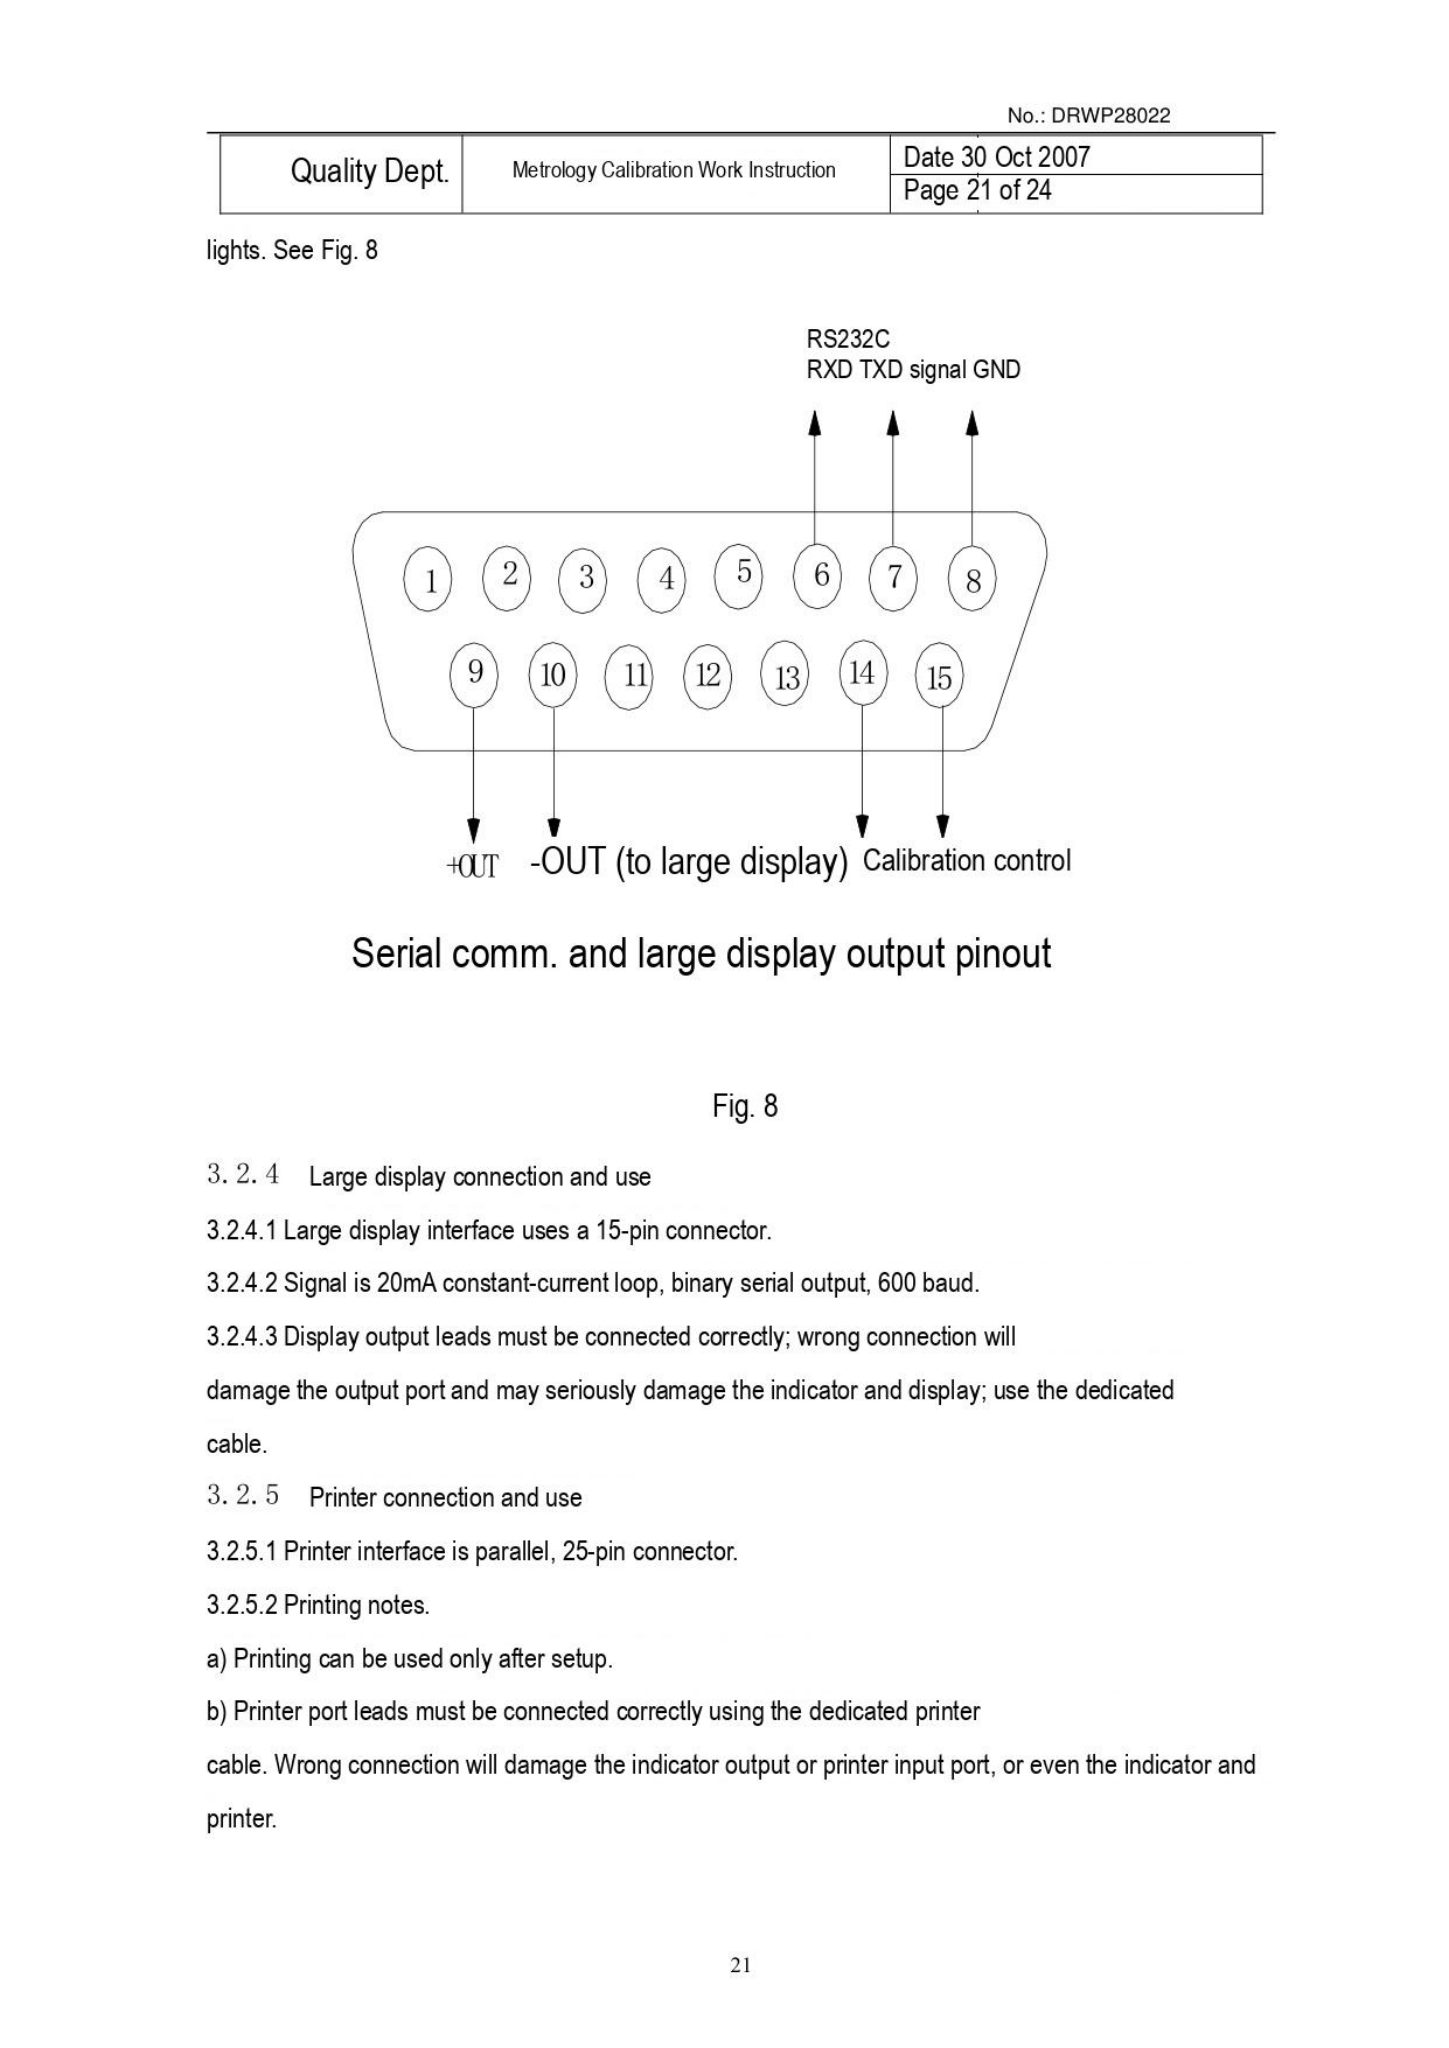No.: DRWP28022

| Quality Dept. | Metrology Calibration Work Instruction | Date 30 Oct 2007 |
|---|---|---|
| | | Page 21 of 24 |

lights. See Fig. 8

RS232C
RXD TXD signal GND

1 2 3 4 5 6 7 8
9 10 11 12 13 14 15

+OUT -OUT (to large display) Calibration control

Serial comm. and large display output pinout

Fig. 8

3. 2. 4 Large display connection and use

3.2.4.1 Large display interface uses a 15-pin connector.

3.2.4.2 Signal is 20mA constant-current loop, binary serial output, 600 baud.

3.2.4.3 Display output leads must be connected correctly; wrong connection will damage the output port and may seriously damage the indicator and display; use the dedicated cable.

3. 2. 5 Printer connection and use

3.2.5.1 Printer interface is parallel, 25-pin connector.

3.2.5.2 Printing notes.

a) Printing can be used only after setup.

b) Printer port leads must be connected correctly using the dedicated printer cable. Wrong connection will damage the indicator output or printer input port, or even the indicator and printer.

21
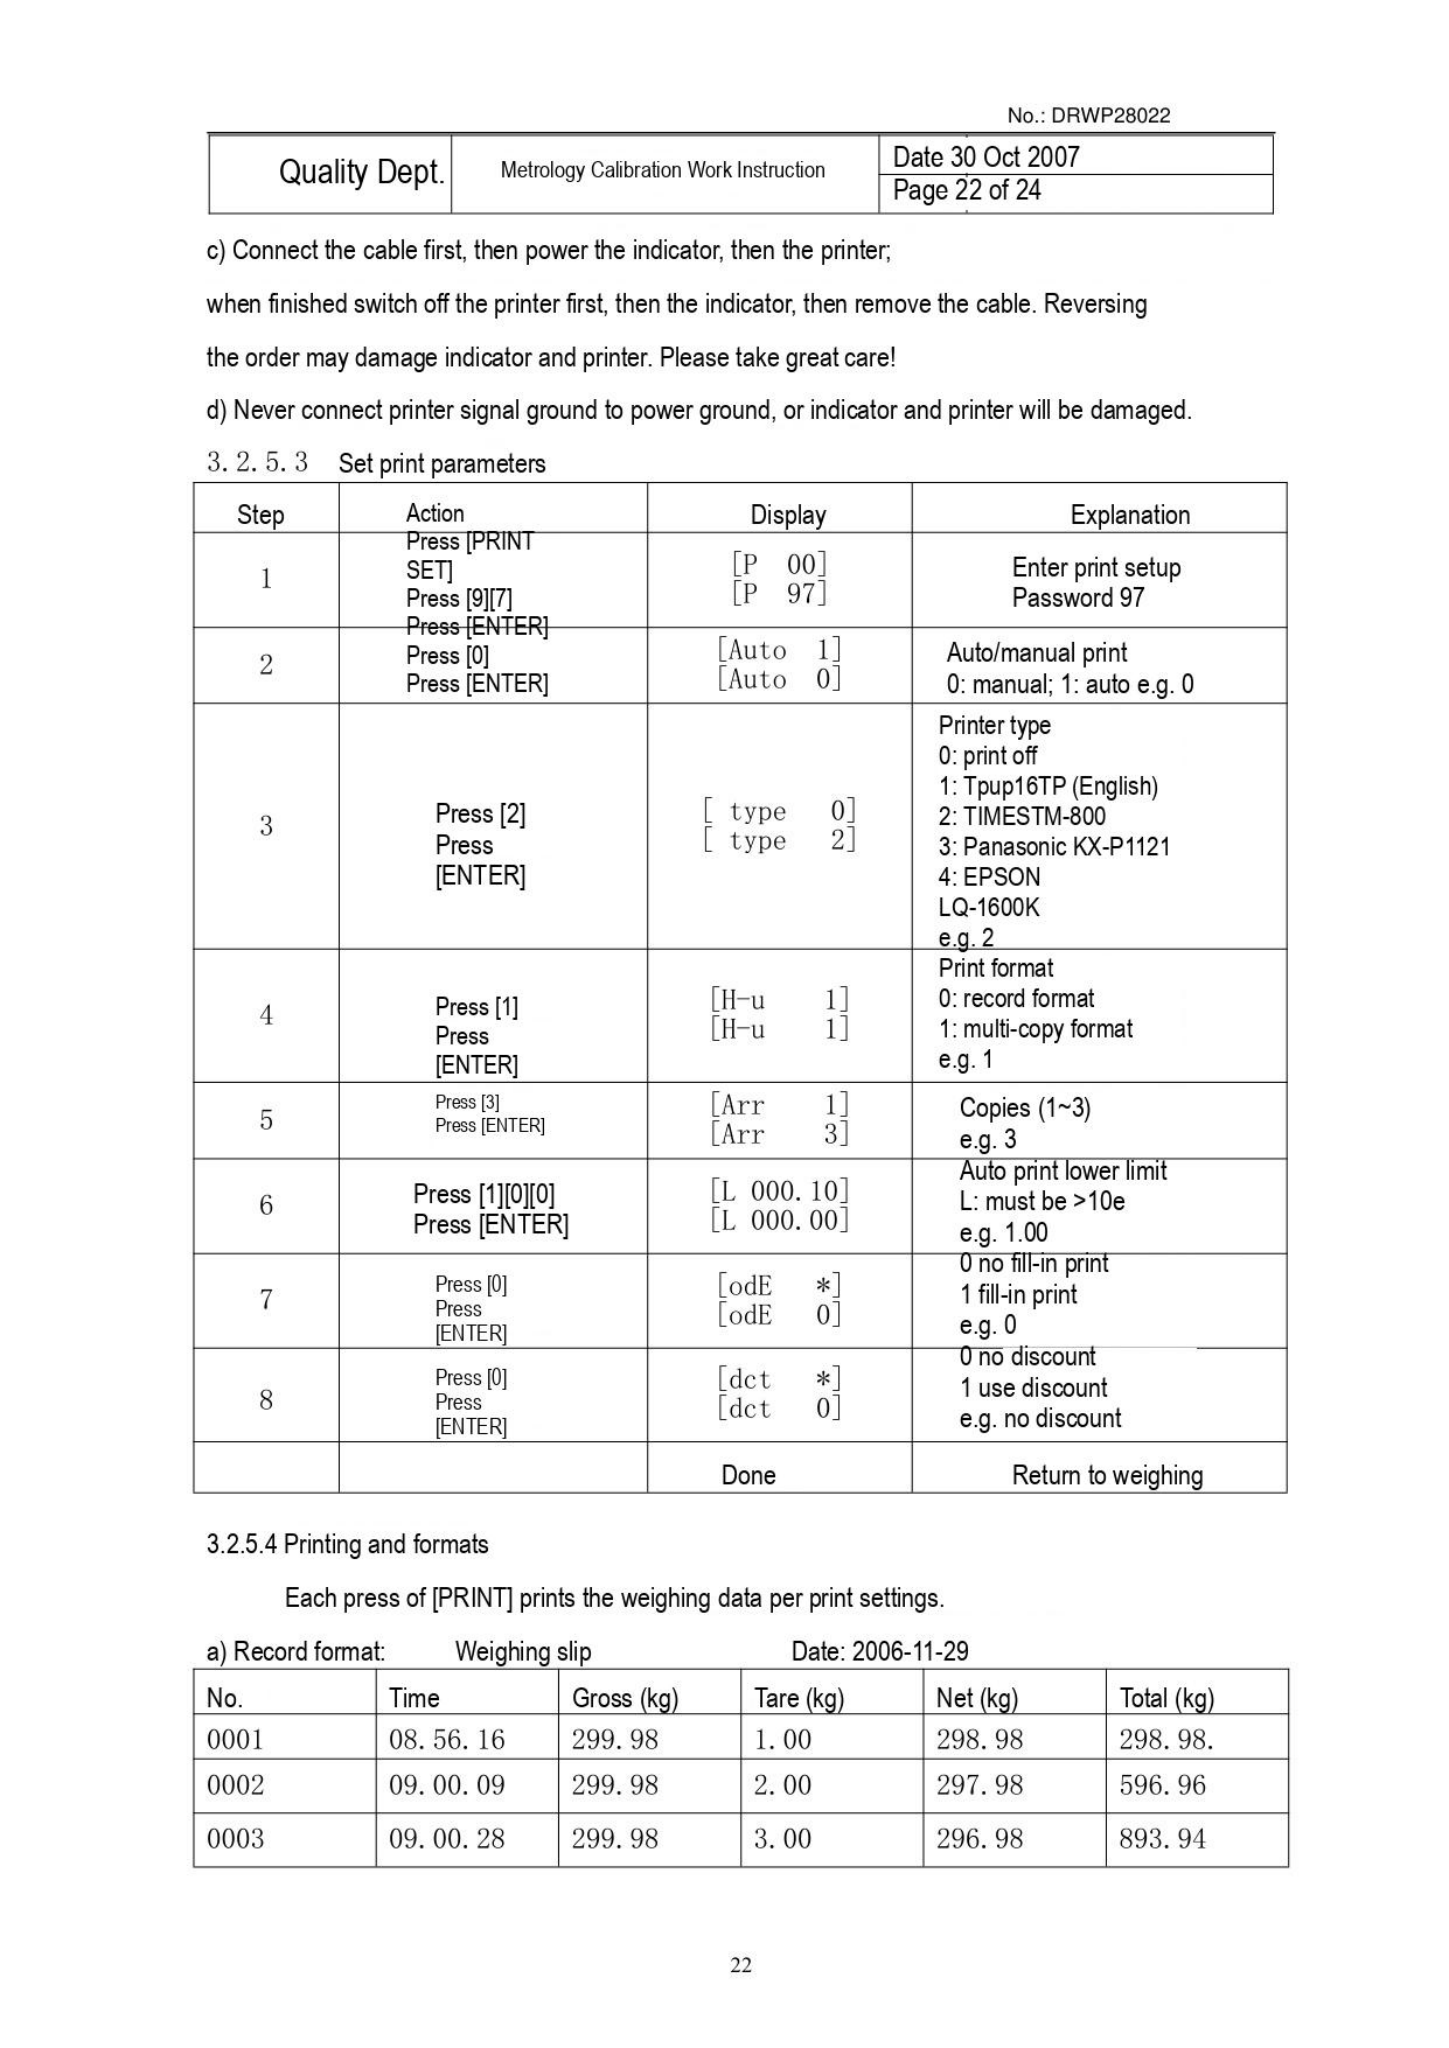No.: DRWP28022

| Quality Dept. | Metrology Calibration Work Instruction | Date 30 Oct 2007<br>Page 22 of 24 |
|---|---|---|

c) Connect the cable first, then power the indicator, then the printer;

when finished switch off the printer first, then the indicator, then remove the cable. Reversing

the order may damage indicator and printer. Please take great care!

d) Never connect printer signal ground to power ground, or indicator and printer will be damaged.

3. 2. 5. 3 Set print parameters

| Step | Action | Display | Explanation |
|---|---|---|---|
| 1 | Press [PRINT SET]<br>Press [9][7]<br>Press [ENTER] | [P 00]<br>[P 97] | Enter print setup<br>Password 97 |
| 2 | Press [0]<br>Press [ENTER] | [Auto 1]<br>[Auto 0] | Auto/manual print<br>0: manual; 1: auto e.g. 0 |
| 3 | Press [2]<br>Press [ENTER] | [ type 0]<br>[ type 2] | Printer type<br>0: print off<br>1: Tpup16TP (English)<br>2: TIMESTM-800<br>3: Panasonic KX-P1121<br>4: EPSON LQ-1600K<br>e.g. 2 |
| 4 | Press [1]<br>Press [ENTER] | [H-u 1]<br>[H-u 1] | Print format<br>0: record format<br>1: multi-copy format<br>e.g. 1 |
| 5 | Press [3]<br>Press [ENTER] | [Arr 1]<br>[Arr 3] | Copies (1~3)<br>e.g. 3 |
| 6 | Press [1][0][0]<br>Press [ENTER] | [L 000. 10]<br>[L 000. 00] | Auto print lower limit<br>L: must be >10e<br>e.g. 1.00 |
| 7 | Press [0]<br>Press [ENTER] | [odE *]<br>[odE 0] | 0 no fill-in print<br>1 fill-in print<br>e.g. 0 |
| 8 | Press [0]<br>Press [ENTER] | [dct *]<br>[dct 0] | 0 no discount<br>1 use discount<br>e.g. no discount |
| | | Done | Return to weighing |

3.2.5.4 Printing and formats

Each press of [PRINT] prints the weighing data per print settings.

a) Record format: Weighing slip Date: 2006-11-29

| No. | Time | Gross (kg) | Tare (kg) | Net (kg) | Total (kg) |
|---|---|---|---|---|---|
| 0001 | 08. 56. 16 | 299. 98 | 1. 00 | 298. 98 | 298. 98. |
| 0002 | 09. 00. 09 | 299. 98 | 2. 00 | 297. 98 | 596. 96 |
| 0003 | 09. 00. 28 | 299. 98 | 3. 00 | 296. 98 | 893. 94 |

22
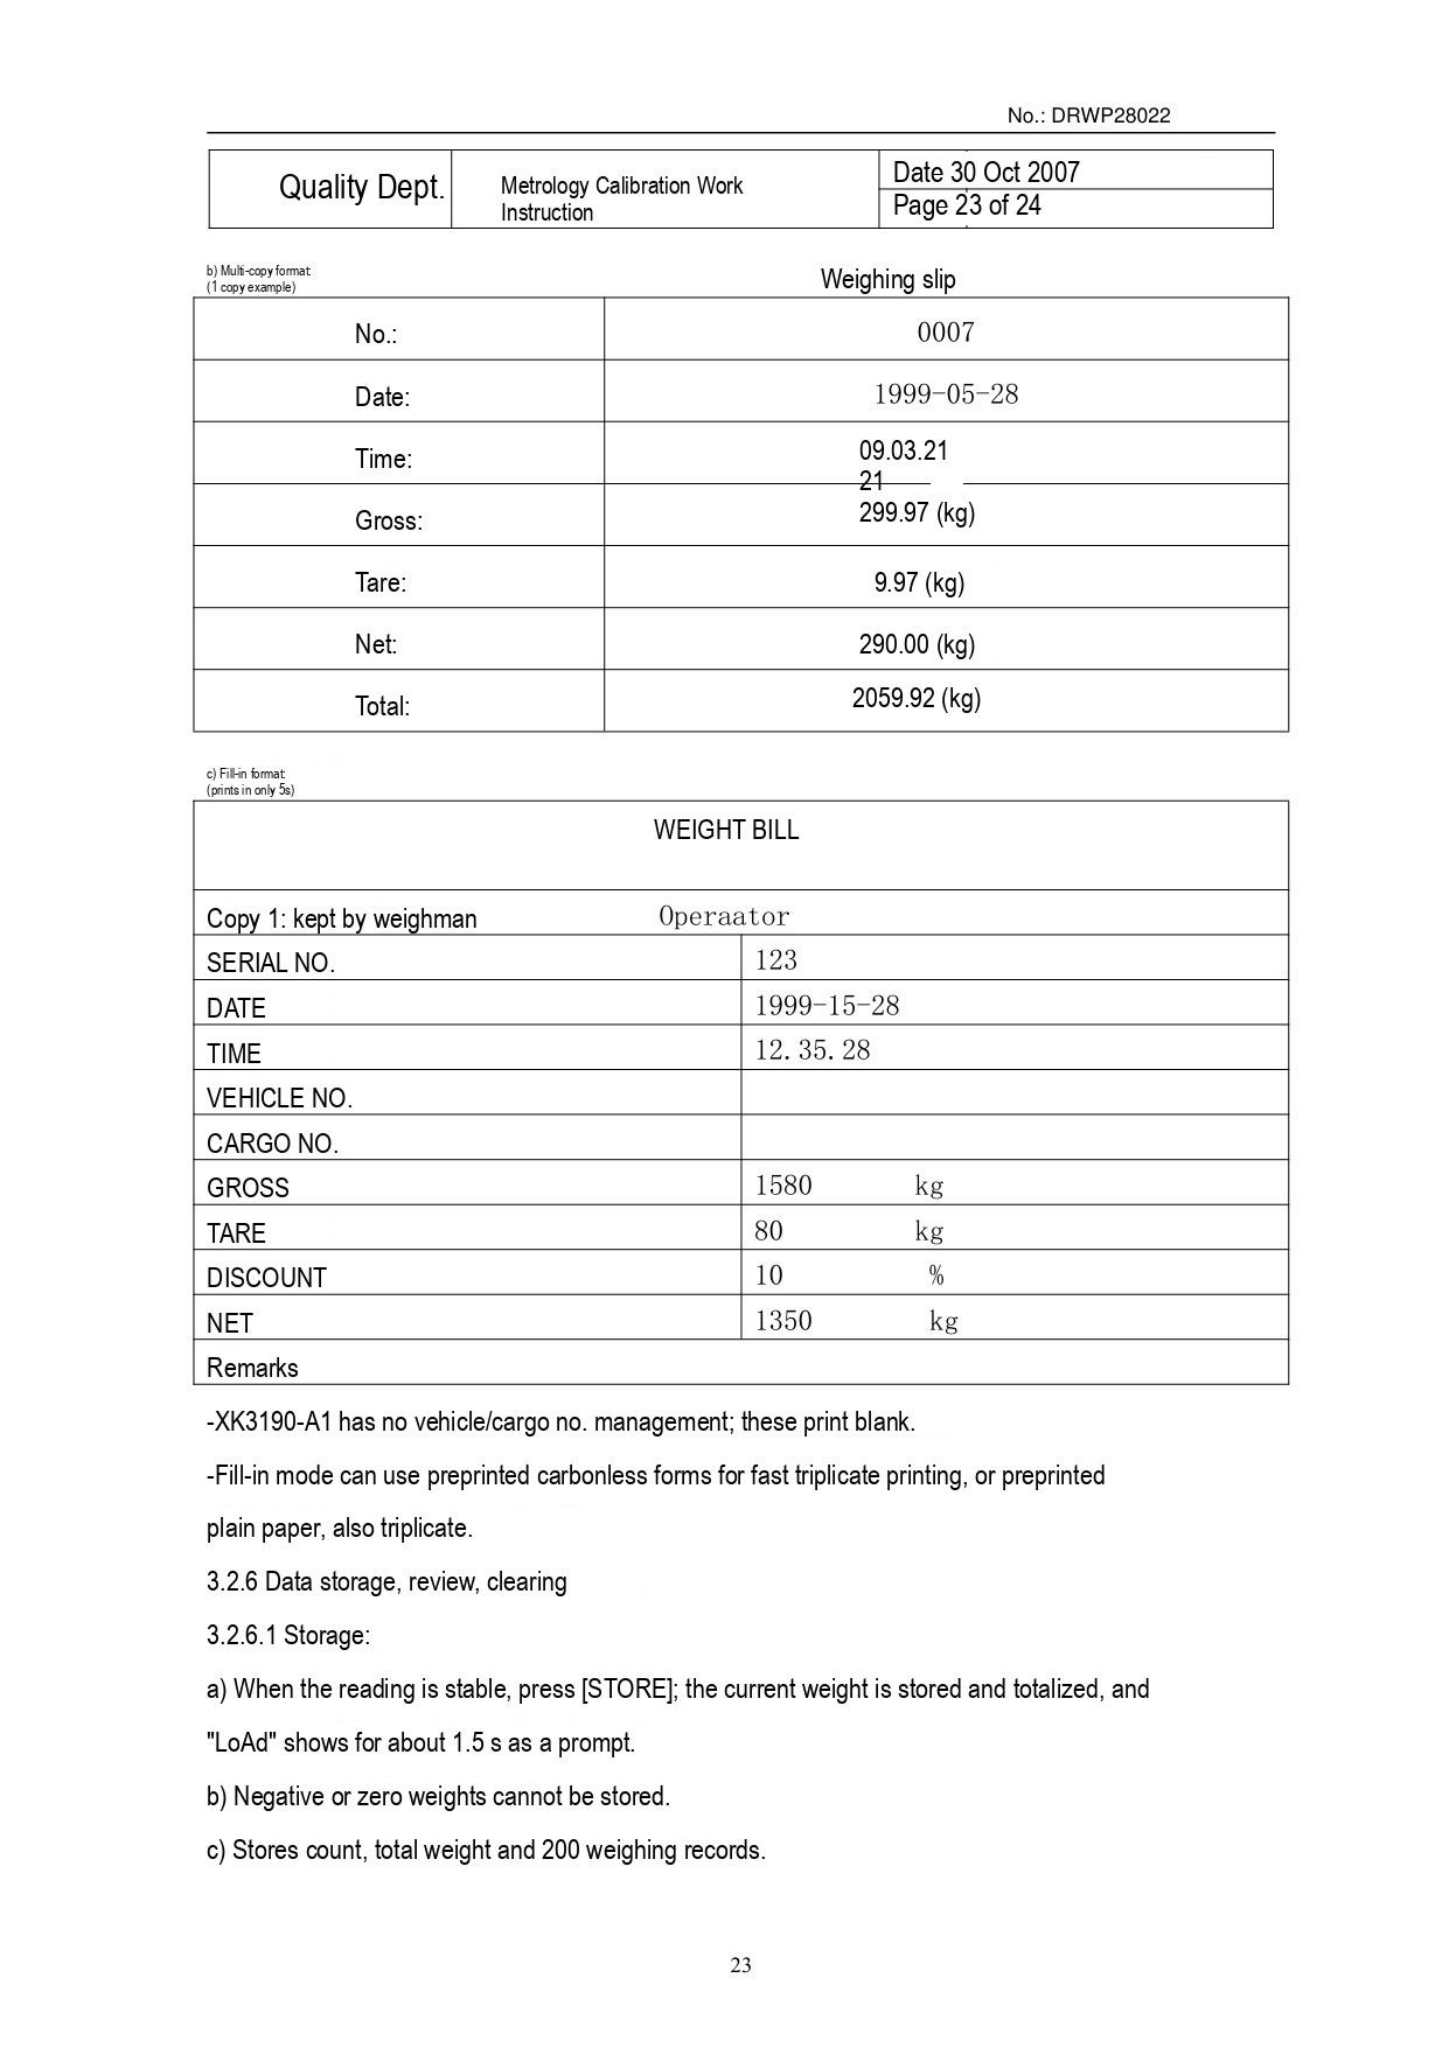No.: DRWP28022

| Quality Dept. | Metrology Calibration Work Instruction | Date 30 Oct 2007 |
|---|---|---|
| | | Page 23 of 24 |

b) Multi-copy format
(1 copy example)

Weighing slip

| No.: | 0007 |
|---|---|
| Date: | 1999-05-28 |
| Time: | 09.03.21 21 |
| Gross: | 299.97 (kg) |
| Tare: | 9.97 (kg) |
| Net: | 290.00 (kg) |
| Total: | 2059.92 (kg) |

c) Fill-in format
(prints in only 5s)

| WEIGHT BILL | |
|---|---|
| Copy 1: kept by weighman | Operaator |
| SERIAL NO. | 123 |
| DATE | 1999-15-28 |
| TIME | 12. 35. 28 |
| VEHICLE NO. | |
| CARGO NO. | |
| GROSS | 1580 kg |
| TARE | 80 kg |
| DISCOUNT | 10 % |
| NET | 1350 kg |
| Remarks | |

-XK3190-A1 has no vehicle/cargo no. management; these print blank.

-Fill-in mode can use preprinted carbonless forms for fast triplicate printing, or preprinted plain paper, also triplicate.

3.2.6 Data storage, review, clearing

3.2.6.1 Storage:

a) When the reading is stable, press [STORE]; the current weight is stored and totalized, and "LoAd" shows for about 1.5 s as a prompt.

b) Negative or zero weights cannot be stored.

c) Stores count, total weight and 200 weighing records.

23
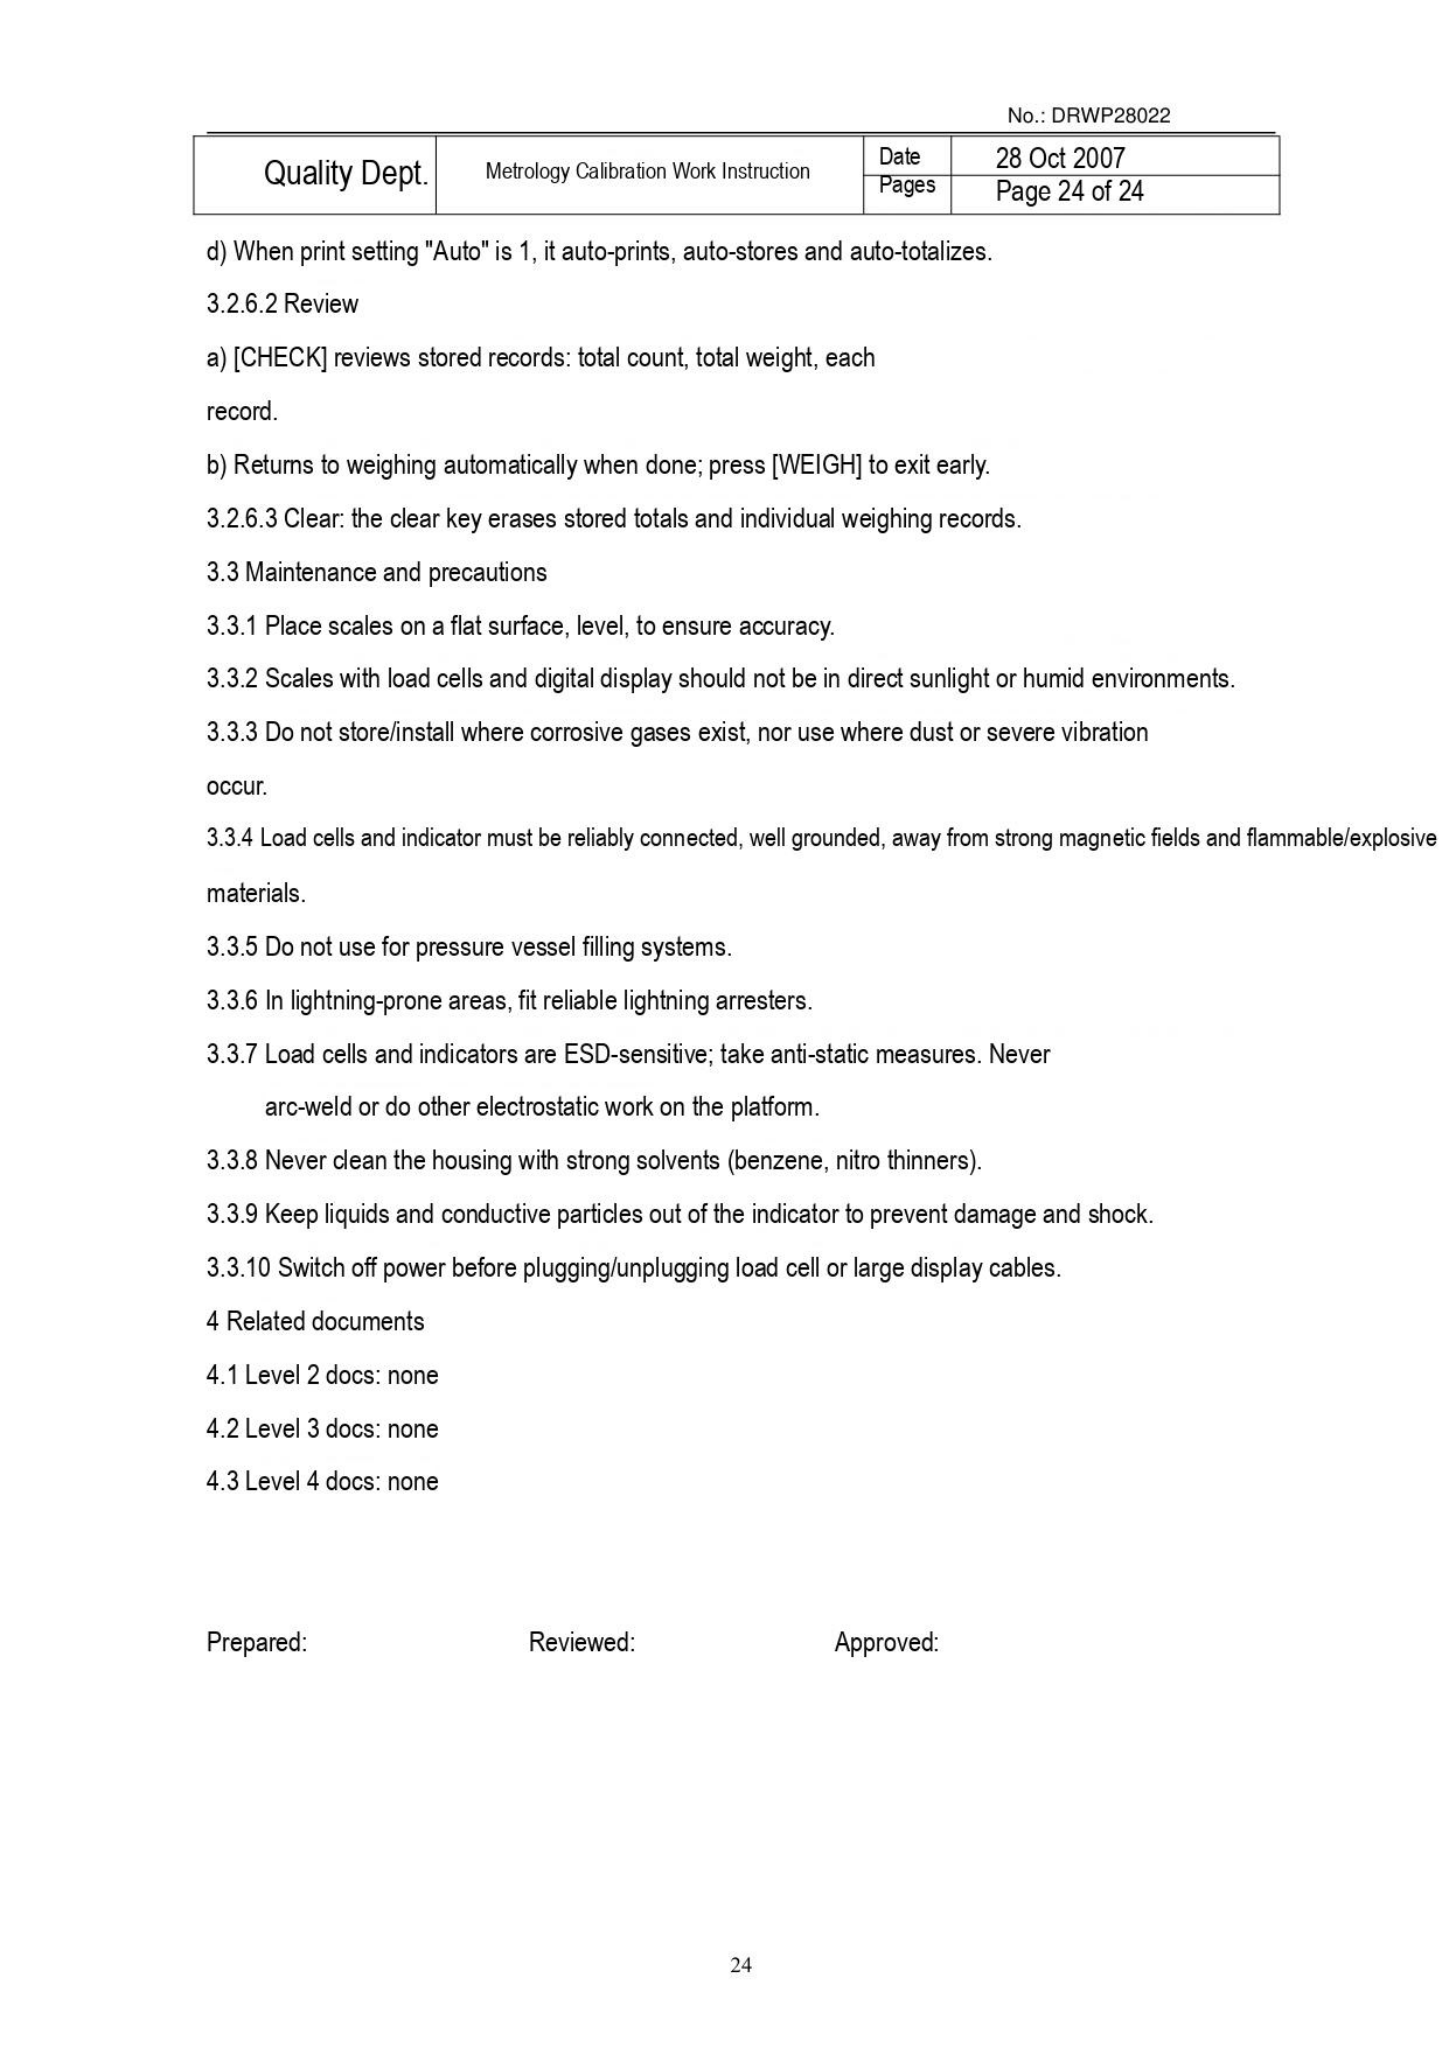No.: DRWP28022

| Quality Dept. | Metrology Calibration Work Instruction | Date | 28 Oct 2007 |
|---|---|---|---|
| | | Pages | Page 24 of 24 |

d) When print setting "Auto" is 1, it auto-prints, auto-stores and auto-totalizes.

3.2.6.2 Review

a) [CHECK] reviews stored records: total count, total weight, each record.

b) Returns to weighing automatically when done; press [WEIGH] to exit early.

3.2.6.3 Clear: the clear key erases stored totals and individual weighing records.

3.3 Maintenance and precautions

3.3.1 Place scales on a flat surface, level, to ensure accuracy.

3.3.2 Scales with load cells and digital display should not be in direct sunlight or humid environments.

3.3.3 Do not store/install where corrosive gases exist, nor use where dust or severe vibration occur.

3.3.4 Load cells and indicator must be reliably connected, well grounded, away from strong magnetic fields and flammable/explosive materials.

3.3.5 Do not use for pressure vessel filling systems.

3.3.6 In lightning-prone areas, fit reliable lightning arresters.

3.3.7 Load cells and indicators are ESD-sensitive; take anti-static measures. Never arc-weld or do other electrostatic work on the platform.

3.3.8 Never clean the housing with strong solvents (benzene, nitro thinners).

3.3.9 Keep liquids and conductive particles out of the indicator to prevent damage and shock.

3.3.10 Switch off power before plugging/unplugging load cell or large display cables.

4 Related documents

4.1 Level 2 docs: none

4.2 Level 3 docs: none

4.3 Level 4 docs: none

Prepared: Reviewed: Approved:

24